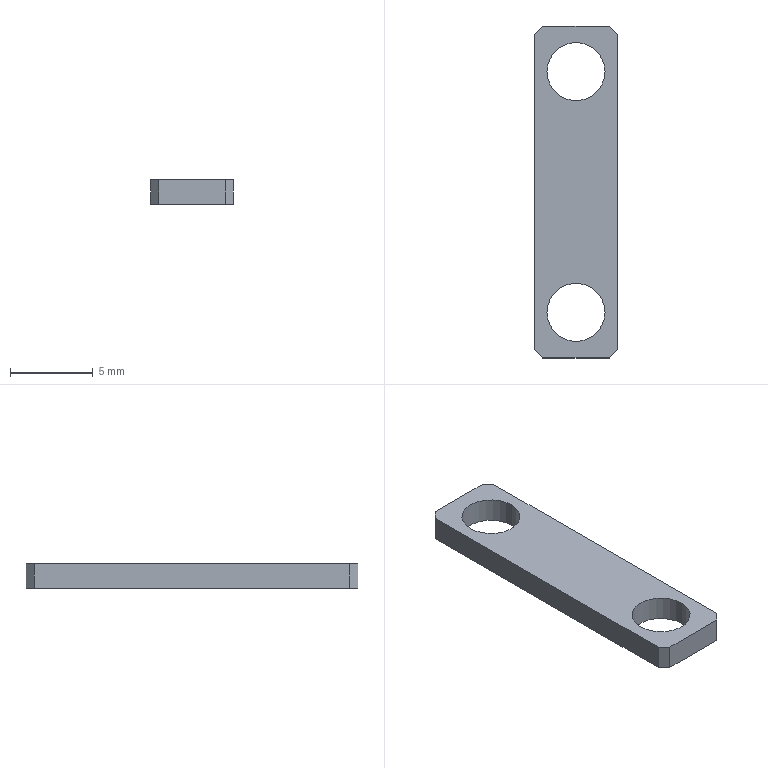Part | NX | features BREP 1 | 1 solid | 14 faces | box 5 x 20 x 1.5 mm | volume 120.387 mm3 | plane 10 | cylinder 4 | commonest cylinder face diameters 3.5 x4
STEP:
#1=CARTESIAN_POINT('',(-1.75,-7.25,0.));
#2=VERTEX_POINT('',#1);
#3=CARTESIAN_POINT('',(1.75,-7.25,0.));
#4=VERTEX_POINT('',#3);
#5=CARTESIAN_POINT('',(0.,-7.25,0.));
#6=DIRECTION('',(0.,0.,1.));
#7=DIRECTION('',(1.,0.,0.));
#8=AXIS2_PLACEMENT_3D('',#5,#6,#7);
#9=CIRCLE('',#8,1.75);
#10=EDGE_CURVE('',#2,#4,#9,.T.);
#11=ORIENTED_EDGE('',*,*,#10,.F.);
#12=CARTESIAN_POINT('',(-1.75,-7.25,1.5));
#13=VERTEX_POINT('',#12);
#14=CARTESIAN_POINT('',(-1.75,-7.25,-0.5));
#15=DIRECTION('',(0.,0.,1.));
#16=VECTOR('',#15,1000.);
#17=LINE('',#14,#16);
#18=EDGE_CURVE('',#13,#2,#17,.F.);
#19=ORIENTED_EDGE('',*,*,#18,.F.);
#20=CARTESIAN_POINT('',(1.75,-7.25,1.5));
#21=VERTEX_POINT('',#20);
#22=CARTESIAN_POINT('',(0.,-7.25,1.5));
#23=DIRECTION('',(0.,0.,1.));
#24=DIRECTION('',(1.,0.,0.));
#25=AXIS2_PLACEMENT_3D('',#22,#23,#24);
#26=CIRCLE('',#25,1.75);
#27=EDGE_CURVE('',#13,#21,#26,.T.);
#28=ORIENTED_EDGE('',*,*,#27,.T.);
#29=CARTESIAN_POINT('',(1.75,-7.25,-0.5));
#30=DIRECTION('',(0.,0.,1.));
#31=VECTOR('',#30,1000.);
#32=LINE('',#29,#31);
#33=EDGE_CURVE('',#21,#4,#32,.F.);
#34=ORIENTED_EDGE('',*,*,#33,.T.);
#35=EDGE_LOOP('',(#11,#19,#28,#34));
#36=FACE_BOUND('',#35,.T.);
#37=CARTESIAN_POINT('',(0.,-7.25,-0.5));
#38=DIRECTION('',(0.,0.,1.));
#39=DIRECTION('',(1.,0.,0.));
#40=AXIS2_PLACEMENT_3D('',#37,#38,#39);
#41=CYLINDRICAL_SURFACE('',#40,1.75);
#42=ADVANCED_FACE('',(#36),#41,.F.);
#43=CARTESIAN_POINT('',(-1.75,7.25,0.));
#44=VERTEX_POINT('',#43);
#45=CARTESIAN_POINT('',(1.75,7.25,0.));
#46=VERTEX_POINT('',#45);
#47=CARTESIAN_POINT('',(0.,7.25,0.));
#48=DIRECTION('',(0.,0.,1.));
#49=DIRECTION('',(1.,0.,0.));
#50=AXIS2_PLACEMENT_3D('',#47,#48,#49);
#51=CIRCLE('',#50,1.75);
#52=EDGE_CURVE('',#44,#46,#51,.T.);
#53=ORIENTED_EDGE('',*,*,#52,.F.);
#54=CARTESIAN_POINT('',(-1.75,7.25,1.5));
#55=VERTEX_POINT('',#54);
#56=CARTESIAN_POINT('',(-1.75,7.25,-0.5));
#57=DIRECTION('',(0.,0.,1.));
#58=VECTOR('',#57,1000.);
#59=LINE('',#56,#58);
#60=EDGE_CURVE('',#55,#44,#59,.F.);
#61=ORIENTED_EDGE('',*,*,#60,.F.);
#62=CARTESIAN_POINT('',(1.75,7.25,1.5));
#63=VERTEX_POINT('',#62);
#64=CARTESIAN_POINT('',(0.,7.25,1.5));
#65=DIRECTION('',(0.,0.,1.));
#66=DIRECTION('',(1.,0.,0.));
#67=AXIS2_PLACEMENT_3D('',#64,#65,#66);
#68=CIRCLE('',#67,1.75);
#69=EDGE_CURVE('',#55,#63,#68,.T.);
#70=ORIENTED_EDGE('',*,*,#69,.T.);
#71=CARTESIAN_POINT('',(1.75,7.25,-0.5));
#72=DIRECTION('',(0.,0.,1.));
#73=VECTOR('',#72,1000.);
#74=LINE('',#71,#73);
#75=EDGE_CURVE('',#63,#46,#74,.F.);
#76=ORIENTED_EDGE('',*,*,#75,.T.);
#77=EDGE_LOOP('',(#53,#61,#70,#76));
#78=FACE_BOUND('',#77,.T.);
#79=CARTESIAN_POINT('',(0.,7.25,-0.5));
#80=DIRECTION('',(0.,0.,1.));
#81=DIRECTION('',(1.,0.,0.));
#82=AXIS2_PLACEMENT_3D('',#79,#80,#81);
#83=CYLINDRICAL_SURFACE('',#82,1.75);
#84=ADVANCED_FACE('',(#78),#83,.F.);
#85=CARTESIAN_POINT('',(2.5,-9.5,1.5));
#86=VERTEX_POINT('',#85);
#87=CARTESIAN_POINT('',(2.5,9.5,1.5));
#88=VERTEX_POINT('',#87);
#89=CARTESIAN_POINT('',(2.5,10.,1.5));
#90=DIRECTION('',(0.,1.,0.));
#91=VECTOR('',#90,1000.);
#92=LINE('',#89,#91);
#93=EDGE_CURVE('',#86,#88,#92,.T.);
#94=ORIENTED_EDGE('',*,*,#93,.F.);
#95=CARTESIAN_POINT('',(2.5,-9.5,0.));
#96=VERTEX_POINT('',#95);
#97=CARTESIAN_POINT('',(2.5,-9.5,1.5));
#98=DIRECTION('',(0.,0.,-1.));
#99=VECTOR('',#98,1000.);
#100=LINE('',#97,#99);
#101=EDGE_CURVE('',#86,#96,#100,.T.);
#102=ORIENTED_EDGE('',*,*,#101,.T.);
#103=CARTESIAN_POINT('',(2.5,9.5,0.));
#104=VERTEX_POINT('',#103);
#105=CARTESIAN_POINT('',(2.5,10.,0.));
#106=DIRECTION('',(0.,1.,0.));
#107=VECTOR('',#106,1000.);
#108=LINE('',#105,#107);
#109=EDGE_CURVE('',#96,#104,#108,.T.);
#110=ORIENTED_EDGE('',*,*,#109,.T.);
#111=CARTESIAN_POINT('',(2.5,9.5,1.5));
#112=DIRECTION('',(0.,0.,1.));
#113=VECTOR('',#112,1000.);
#114=LINE('',#111,#113);
#115=EDGE_CURVE('',#104,#88,#114,.T.);
#116=ORIENTED_EDGE('',*,*,#115,.T.);
#117=EDGE_LOOP('',(#94,#102,#110,#116));
#118=FACE_BOUND('',#117,.T.);
#119=CARTESIAN_POINT('',(2.5,10.,1.5));
#120=DIRECTION('',(-1.,0.,0.));
#121=DIRECTION('',(0.,1.,0.));
#122=AXIS2_PLACEMENT_3D('',#119,#120,#121);
#123=PLANE('',#122);
#124=ADVANCED_FACE('',(#118),#123,.F.);
#125=CARTESIAN_POINT('',(2.,10.,0.));
#126=VERTEX_POINT('',#125);
#127=CARTESIAN_POINT('',(-2.,10.,0.));
#128=VERTEX_POINT('',#127);
#129=CARTESIAN_POINT('',(-2.5,10.,0.));
#130=DIRECTION('',(-1.,0.,0.));
#131=VECTOR('',#130,1000.);
#132=LINE('',#129,#131);
#133=EDGE_CURVE('',#126,#128,#132,.T.);
#134=ORIENTED_EDGE('',*,*,#133,.T.);
#135=CARTESIAN_POINT('',(-2.,10.,1.5));
#136=VERTEX_POINT('',#135);
#137=CARTESIAN_POINT('',(-2.,10.,1.5));
#138=DIRECTION('',(0.,0.,1.));
#139=VECTOR('',#138,1000.);
#140=LINE('',#137,#139);
#141=EDGE_CURVE('',#128,#136,#140,.T.);
#142=ORIENTED_EDGE('',*,*,#141,.T.);
#143=CARTESIAN_POINT('',(2.,10.,1.5));
#144=VERTEX_POINT('',#143);
#145=CARTESIAN_POINT('',(-2.5,10.,1.5));
#146=DIRECTION('',(-1.,0.,0.));
#147=VECTOR('',#146,1000.);
#148=LINE('',#145,#147);
#149=EDGE_CURVE('',#144,#136,#148,.T.);
#150=ORIENTED_EDGE('',*,*,#149,.F.);
#151=CARTESIAN_POINT('',(2.,10.,1.5));
#152=DIRECTION('',(0.,0.,-1.));
#153=VECTOR('',#152,1000.);
#154=LINE('',#151,#153);
#155=EDGE_CURVE('',#144,#126,#154,.T.);
#156=ORIENTED_EDGE('',*,*,#155,.T.);
#157=EDGE_LOOP('',(#134,#142,#150,#156));
#158=FACE_BOUND('',#157,.T.);
#159=CARTESIAN_POINT('',(-2.5,10.,1.5));
#160=DIRECTION('',(0.,-1.,0.));
#161=DIRECTION('',(0.,0.,-1.));
#162=AXIS2_PLACEMENT_3D('',#159,#160,#161);
#163=PLANE('',#162);
#164=ADVANCED_FACE('',(#158),#163,.F.);
#165=CARTESIAN_POINT('',(-2.5,9.5,0.));
#166=VERTEX_POINT('',#165);
#167=CARTESIAN_POINT('',(-2.5,-9.5,0.));
#168=VERTEX_POINT('',#167);
#169=CARTESIAN_POINT('',(-2.5,10.,0.));
#170=DIRECTION('',(0.,-1.,0.));
#171=VECTOR('',#170,1000.);
#172=LINE('',#169,#171);
#173=EDGE_CURVE('',#166,#168,#172,.T.);
#174=ORIENTED_EDGE('',*,*,#173,.T.);
#175=CARTESIAN_POINT('',(-2.5,-9.5,1.5));
#176=VERTEX_POINT('',#175);
#177=CARTESIAN_POINT('',(-2.5,-9.5,1.5));
#178=DIRECTION('',(0.,0.,1.));
#179=VECTOR('',#178,1000.);
#180=LINE('',#177,#179);
#181=EDGE_CURVE('',#168,#176,#180,.T.);
#182=ORIENTED_EDGE('',*,*,#181,.T.);
#183=CARTESIAN_POINT('',(-2.5,9.5,1.5));
#184=VERTEX_POINT('',#183);
#185=CARTESIAN_POINT('',(-2.5,10.,1.5));
#186=DIRECTION('',(0.,-1.,0.));
#187=VECTOR('',#186,1000.);
#188=LINE('',#185,#187);
#189=EDGE_CURVE('',#184,#176,#188,.T.);
#190=ORIENTED_EDGE('',*,*,#189,.F.);
#191=CARTESIAN_POINT('',(-2.5,9.5,1.5));
#192=DIRECTION('',(0.,0.,-1.));
#193=VECTOR('',#192,1000.);
#194=LINE('',#191,#193);
#195=EDGE_CURVE('',#184,#166,#194,.T.);
#196=ORIENTED_EDGE('',*,*,#195,.T.);
#197=EDGE_LOOP('',(#174,#182,#190,#196));
#198=FACE_BOUND('',#197,.T.);
#199=CARTESIAN_POINT('',(-2.5,10.,1.5));
#200=DIRECTION('',(1.,0.,0.));
#201=DIRECTION('',(0.,1.,0.));
#202=AXIS2_PLACEMENT_3D('',#199,#200,#201);
#203=PLANE('',#202);
#204=ADVANCED_FACE('',(#198),#203,.F.);
#205=CARTESIAN_POINT('',(-2.,-10.,0.));
#206=VERTEX_POINT('',#205);
#207=CARTESIAN_POINT('',(2.,-10.,0.));
#208=VERTEX_POINT('',#207);
#209=CARTESIAN_POINT('',(-2.5,-10.,0.));
#210=DIRECTION('',(1.,0.,0.));
#211=VECTOR('',#210,1000.);
#212=LINE('',#209,#211);
#213=EDGE_CURVE('',#206,#208,#212,.T.);
#214=ORIENTED_EDGE('',*,*,#213,.T.);
#215=CARTESIAN_POINT('',(2.,-10.,1.5));
#216=VERTEX_POINT('',#215);
#217=CARTESIAN_POINT('',(2.,-10.,1.5));
#218=DIRECTION('',(0.,0.,1.));
#219=VECTOR('',#218,1000.);
#220=LINE('',#217,#219);
#221=EDGE_CURVE('',#208,#216,#220,.T.);
#222=ORIENTED_EDGE('',*,*,#221,.T.);
#223=CARTESIAN_POINT('',(-2.,-10.,1.5));
#224=VERTEX_POINT('',#223);
#225=CARTESIAN_POINT('',(-2.5,-10.,1.5));
#226=DIRECTION('',(1.,0.,0.));
#227=VECTOR('',#226,1000.);
#228=LINE('',#225,#227);
#229=EDGE_CURVE('',#224,#216,#228,.T.);
#230=ORIENTED_EDGE('',*,*,#229,.F.);
#231=CARTESIAN_POINT('',(-2.,-10.,1.5));
#232=DIRECTION('',(0.,0.,-1.));
#233=VECTOR('',#232,1000.);
#234=LINE('',#231,#233);
#235=EDGE_CURVE('',#224,#206,#234,.T.);
#236=ORIENTED_EDGE('',*,*,#235,.T.);
#237=EDGE_LOOP('',(#214,#222,#230,#236));
#238=FACE_BOUND('',#237,.T.);
#239=CARTESIAN_POINT('',(-2.5,-10.,1.5));
#240=DIRECTION('',(0.,1.,0.));
#241=DIRECTION('',(1.,0.,0.));
#242=AXIS2_PLACEMENT_3D('',#239,#240,#241);
#243=PLANE('',#242);
#244=ADVANCED_FACE('',(#238),#243,.F.);
#245=ORIENTED_EDGE('',*,*,#229,.T.);
#246=CARTESIAN_POINT('',(6.,-6.,1.5));
#247=DIRECTION('',(0.7071,0.7071,0.));
#248=VECTOR('',#247,1000.);
#249=LINE('',#246,#248);
#250=EDGE_CURVE('',#216,#86,#249,.T.);
#251=ORIENTED_EDGE('',*,*,#250,.T.);
#252=ORIENTED_EDGE('',*,*,#93,.T.);
#253=CARTESIAN_POINT('',(6.,6.,1.5));
#254=DIRECTION('',(-0.7071,0.7071,0.));
#255=VECTOR('',#254,1000.);
#256=LINE('',#253,#255);
#257=EDGE_CURVE('',#88,#144,#256,.T.);
#258=ORIENTED_EDGE('',*,*,#257,.T.);
#259=ORIENTED_EDGE('',*,*,#149,.T.);
#260=CARTESIAN_POINT('',(-6.,6.,1.5));
#261=DIRECTION('',(-0.7071,-0.7071,0.));
#262=VECTOR('',#261,1000.);
#263=LINE('',#260,#262);
#264=EDGE_CURVE('',#136,#184,#263,.T.);
#265=ORIENTED_EDGE('',*,*,#264,.T.);
#266=ORIENTED_EDGE('',*,*,#189,.T.);
#267=CARTESIAN_POINT('',(-6.,-6.,1.5));
#268=DIRECTION('',(0.7071,-0.7071,0.));
#269=VECTOR('',#268,1000.);
#270=LINE('',#267,#269);
#271=EDGE_CURVE('',#176,#224,#270,.T.);
#272=ORIENTED_EDGE('',*,*,#271,.T.);
#273=EDGE_LOOP('',(#245,#251,#252,#258,#259,#265,#266,#272));
#274=FACE_BOUND('',#273,.T.);
#275=CARTESIAN_POINT('',(0.,-7.25,1.5));
#276=DIRECTION('',(0.,0.,1.));
#277=DIRECTION('',(1.,0.,0.));
#278=AXIS2_PLACEMENT_3D('',#275,#276,#277);
#279=CIRCLE('',#278,1.75);
#280=EDGE_CURVE('',#21,#13,#279,.T.);
#281=ORIENTED_EDGE('',*,*,#280,.F.);
#282=ORIENTED_EDGE('',*,*,#27,.F.);
#283=EDGE_LOOP('',(#281,#282));
#284=FACE_BOUND('',#283,.T.);
#285=CARTESIAN_POINT('',(0.,7.25,1.5));
#286=DIRECTION('',(0.,0.,1.));
#287=DIRECTION('',(1.,0.,0.));
#288=AXIS2_PLACEMENT_3D('',#285,#286,#287);
#289=CIRCLE('',#288,1.75);
#290=EDGE_CURVE('',#63,#55,#289,.T.);
#291=ORIENTED_EDGE('',*,*,#290,.F.);
#292=ORIENTED_EDGE('',*,*,#69,.F.);
#293=EDGE_LOOP('',(#291,#292));
#294=FACE_BOUND('',#293,.T.);
#295=CARTESIAN_POINT('',(0.,0.,1.5));
#296=DIRECTION('',(0.,0.,1.));
#297=DIRECTION('',(1.,0.,0.));
#298=AXIS2_PLACEMENT_3D('',#295,#296,#297);
#299=PLANE('',#298);
#300=ADVANCED_FACE('',(#274,#284,#294),#299,.T.);
#301=ORIENTED_EDGE('',*,*,#109,.F.);
#302=CARTESIAN_POINT('',(2.5,-9.5,0.));
#303=DIRECTION('',(-0.7071,-0.7071,0.));
#304=VECTOR('',#303,1000.);
#305=LINE('',#302,#304);
#306=EDGE_CURVE('',#96,#208,#305,.T.);
#307=ORIENTED_EDGE('',*,*,#306,.T.);
#308=ORIENTED_EDGE('',*,*,#213,.F.);
#309=CARTESIAN_POINT('',(-2.,-10.,0.));
#310=DIRECTION('',(-0.7071,0.7071,0.));
#311=VECTOR('',#310,1000.);
#312=LINE('',#309,#311);
#313=EDGE_CURVE('',#206,#168,#312,.T.);
#314=ORIENTED_EDGE('',*,*,#313,.T.);
#315=ORIENTED_EDGE('',*,*,#173,.F.);
#316=CARTESIAN_POINT('',(-2.5,9.5,0.));
#317=DIRECTION('',(0.7071,0.7071,0.));
#318=VECTOR('',#317,1000.);
#319=LINE('',#316,#318);
#320=EDGE_CURVE('',#166,#128,#319,.T.);
#321=ORIENTED_EDGE('',*,*,#320,.T.);
#322=ORIENTED_EDGE('',*,*,#133,.F.);
#323=CARTESIAN_POINT('',(2.,10.,0.));
#324=DIRECTION('',(0.7071,-0.7071,0.));
#325=VECTOR('',#324,1000.);
#326=LINE('',#323,#325);
#327=EDGE_CURVE('',#126,#104,#326,.T.);
#328=ORIENTED_EDGE('',*,*,#327,.T.);
#329=EDGE_LOOP('',(#301,#307,#308,#314,#315,#321,#322,#328));
#330=FACE_BOUND('',#329,.T.);
#331=CARTESIAN_POINT('',(0.,-7.25,0.));
#332=DIRECTION('',(0.,0.,1.));
#333=DIRECTION('',(1.,0.,0.));
#334=AXIS2_PLACEMENT_3D('',#331,#332,#333);
#335=CIRCLE('',#334,1.75);
#336=EDGE_CURVE('',#4,#2,#335,.T.);
#337=ORIENTED_EDGE('',*,*,#336,.T.);
#338=ORIENTED_EDGE('',*,*,#10,.T.);
#339=EDGE_LOOP('',(#337,#338));
#340=FACE_BOUND('',#339,.T.);
#341=CARTESIAN_POINT('',(0.,7.25,0.));
#342=DIRECTION('',(0.,0.,1.));
#343=DIRECTION('',(1.,0.,0.));
#344=AXIS2_PLACEMENT_3D('',#341,#342,#343);
#345=CIRCLE('',#344,1.75);
#346=EDGE_CURVE('',#46,#44,#345,.T.);
#347=ORIENTED_EDGE('',*,*,#346,.T.);
#348=ORIENTED_EDGE('',*,*,#52,.T.);
#349=EDGE_LOOP('',(#347,#348));
#350=FACE_BOUND('',#349,.T.);
#351=CARTESIAN_POINT('',(0.,0.,0.));
#352=DIRECTION('',(0.,0.,1.));
#353=DIRECTION('',(1.,0.,0.));
#354=AXIS2_PLACEMENT_3D('',#351,#352,#353);
#355=PLANE('',#354);
#356=ADVANCED_FACE('',(#330,#340,#350),#355,.F.);
#357=ORIENTED_EDGE('',*,*,#60,.T.);
#358=ORIENTED_EDGE('',*,*,#346,.F.);
#359=ORIENTED_EDGE('',*,*,#75,.F.);
#360=ORIENTED_EDGE('',*,*,#290,.T.);
#361=EDGE_LOOP('',(#357,#358,#359,#360));
#362=FACE_BOUND('',#361,.T.);
#363=CARTESIAN_POINT('',(0.,7.25,-0.5));
#364=DIRECTION('',(0.,0.,1.));
#365=DIRECTION('',(1.,0.,0.));
#366=AXIS2_PLACEMENT_3D('',#363,#364,#365);
#367=CYLINDRICAL_SURFACE('',#366,1.75);
#368=ADVANCED_FACE('',(#362),#367,.F.);
#369=ORIENTED_EDGE('',*,*,#18,.T.);
#370=ORIENTED_EDGE('',*,*,#336,.F.);
#371=ORIENTED_EDGE('',*,*,#33,.F.);
#372=ORIENTED_EDGE('',*,*,#280,.T.);
#373=EDGE_LOOP('',(#369,#370,#371,#372));
#374=FACE_BOUND('',#373,.T.);
#375=CARTESIAN_POINT('',(0.,-7.25,-0.5));
#376=DIRECTION('',(0.,0.,1.));
#377=DIRECTION('',(1.,0.,0.));
#378=AXIS2_PLACEMENT_3D('',#375,#376,#377);
#379=CYLINDRICAL_SURFACE('',#378,1.75);
#380=ADVANCED_FACE('',(#374),#379,.F.);
#381=ORIENTED_EDGE('',*,*,#250,.F.);
#382=ORIENTED_EDGE('',*,*,#221,.F.);
#383=ORIENTED_EDGE('',*,*,#306,.F.);
#384=ORIENTED_EDGE('',*,*,#101,.F.);
#385=EDGE_LOOP('',(#381,#382,#383,#384));
#386=FACE_BOUND('',#385,.T.);
#387=CARTESIAN_POINT('',(2.5,-9.5,1.5));
#388=DIRECTION('',(-0.7071,0.7071,0.));
#389=DIRECTION('',(0.,0.,1.));
#390=AXIS2_PLACEMENT_3D('',#387,#388,#389);
#391=PLANE('',#390);
#392=ADVANCED_FACE('',(#386),#391,.F.);
#393=ORIENTED_EDGE('',*,*,#271,.F.);
#394=ORIENTED_EDGE('',*,*,#181,.F.);
#395=ORIENTED_EDGE('',*,*,#313,.F.);
#396=ORIENTED_EDGE('',*,*,#235,.F.);
#397=EDGE_LOOP('',(#393,#394,#395,#396));
#398=FACE_BOUND('',#397,.T.);
#399=CARTESIAN_POINT('',(-2.,-10.,1.5));
#400=DIRECTION('',(0.7071,0.7071,0.));
#401=DIRECTION('',(0.,0.,-1.));
#402=AXIS2_PLACEMENT_3D('',#399,#400,#401);
#403=PLANE('',#402);
#404=ADVANCED_FACE('',(#398),#403,.F.);
#405=ORIENTED_EDGE('',*,*,#264,.F.);
#406=ORIENTED_EDGE('',*,*,#141,.F.);
#407=ORIENTED_EDGE('',*,*,#320,.F.);
#408=ORIENTED_EDGE('',*,*,#195,.F.);
#409=EDGE_LOOP('',(#405,#406,#407,#408));
#410=FACE_BOUND('',#409,.T.);
#411=CARTESIAN_POINT('',(-2.5,9.5,1.5));
#412=DIRECTION('',(0.7071,-0.7071,0.));
#413=DIRECTION('',(0.,0.,-1.));
#414=AXIS2_PLACEMENT_3D('',#411,#412,#413);
#415=PLANE('',#414);
#416=ADVANCED_FACE('',(#410),#415,.F.);
#417=ORIENTED_EDGE('',*,*,#257,.F.);
#418=ORIENTED_EDGE('',*,*,#115,.F.);
#419=ORIENTED_EDGE('',*,*,#327,.F.);
#420=ORIENTED_EDGE('',*,*,#155,.F.);
#421=EDGE_LOOP('',(#417,#418,#419,#420));
#422=FACE_BOUND('',#421,.T.);
#423=CARTESIAN_POINT('',(2.,10.,1.5));
#424=DIRECTION('',(-0.7071,-0.7071,0.));
#425=DIRECTION('',(-0.7071,0.7071,0.));
#426=AXIS2_PLACEMENT_3D('',#423,#424,#425);
#427=PLANE('',#426);
#428=ADVANCED_FACE('',(#422),#427,.F.);
#429=CLOSED_SHELL('',(#42,#84,#124,#164,#204,#244,#300,#356,#368,#380,#392,#404,#416,#428));
#430=MANIFOLD_SOLID_BREP('',#429);
#431=(LENGTH_UNIT()NAMED_UNIT(*)SI_UNIT(.MILLI.,.METRE.));
#432=UNCERTAINTY_MEASURE_WITH_UNIT(LENGTH_MEASURE(0.00001),#431,'','');
#433=(NAMED_UNIT(*)PLANE_ANGLE_UNIT()SI_UNIT($,.RADIAN.));
#434=(NAMED_UNIT(*)SI_UNIT($,.STERADIAN.)SOLID_ANGLE_UNIT());
#435=(GEOMETRIC_REPRESENTATION_CONTEXT(3)GLOBAL_UNCERTAINTY_ASSIGNED_CONTEXT((#432))GLOBAL_UNIT_ASSIGNED_CONTEXT((#431,#433,#434))REPRESENTATION_CONTEXT('',''));
#436=ADVANCED_BREP_SHAPE_REPRESENTATION('',(#430),#435);